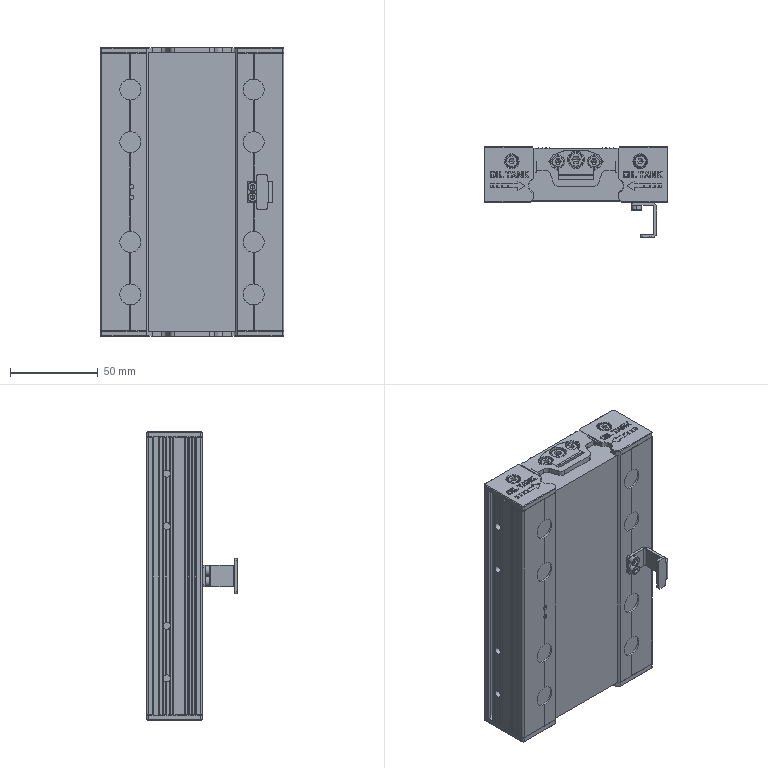Part | SolidWorks | features BaseBody 3 | 3 solids | 2164 faces | box 105 x 52 x 165 mm | volume 515156 mm3 | plane 1293 | cylinder 600 | cone 195 | torus 44 | spline 32 | commonest cylinder face diameters 0.2 x152 0.4 x95 2 x38 4.2 x36 7 x36 8 x25